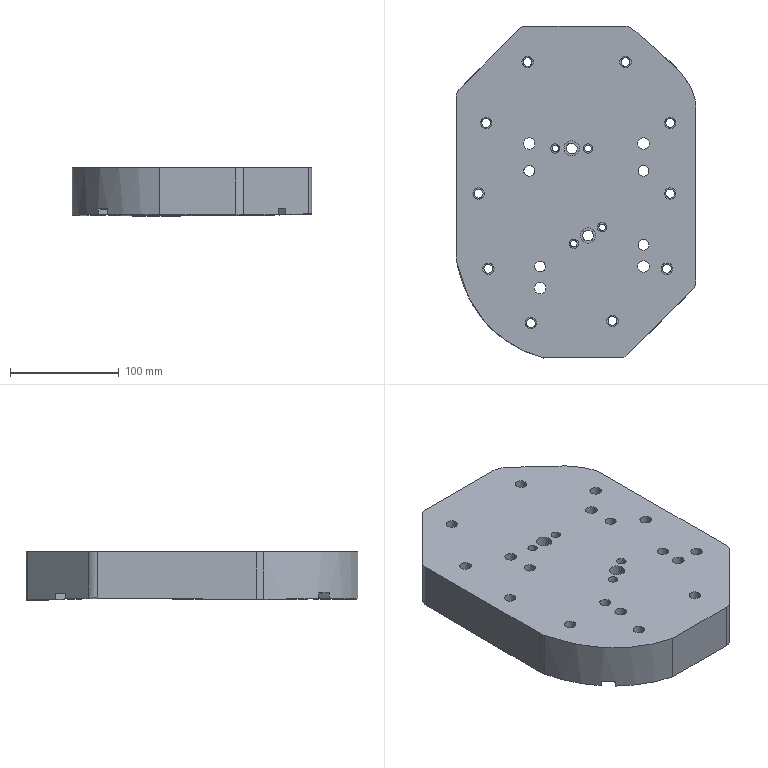Part | STEP file | 815_id1706_x_t | 1 solid | 227 faces | box 220 x 305 x 44.601 mm | volume 2092283 mm3 | spline 124 | cylinder 53 | plane 43 | other 2 | torus 2 | sphere 2 | cone 1 | commonest cylinder face diameters 10.5 x14 8.2 x10 10 x6 20 x5 6.1 x4 8.5 x4